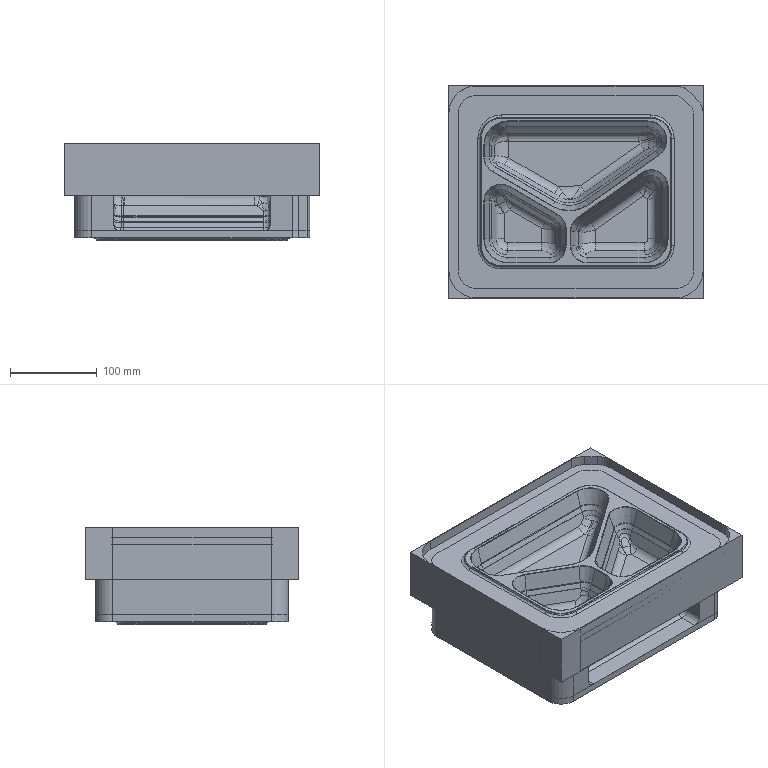NC program | NX | posted with a generic post | part box 295.651 x 246.652 x 112.895 mm
Lines 268779 to 269046 of 299251:
(D4 , TOOL : V2.0)
N537544 M6
N537546 G53
N537548 G17 G0 G90 X123.435 Y60.74 S2000 M3 M8
N537550 G43 Z210.5 H0
N537552 G94 G81 G98 Z46.884 F150. R51.884
N537554 X115.435 Y60.61
N537556 X113.468 Y72.487
N537558 X121.842 Y72.731
N537560 X116.481 Y83.572
N537562 X106.869 Y82.551
N537564 X107.906 Y92.1
N537566 X97.036 Y97.401
N537568 X96.748 Y89.06
N537570 X84.854 Y90.936
N537572 X85.037 Y98.936
N537574 X72.889
N537576 X72.732 Y90.936
N537578 X60.61
N537580 X60.74 Y98.936
N537582 X48.592
N537584 X48.488 Y90.936
N537586 X36.444 Y98.936
N537588 X36.366 Y90.936
N537590 X24.244
N537592 X24.296 Y98.936
N537594 X12.148
N537596 X12.122 Y90.936
N537598 X0.
N537600 Y98.936
N537602 X-12.148
N537604 X-12.122 Y90.936
N537606 X-24.244
N537608 X-24.296 Y98.936
N537610 X-36.444
N537612 X-36.366 Y90.936
N537614 X-48.488
N537616 X-48.592 Y98.936
N537618 X-60.74
N537620 X-72.889
N537622 X-85.037
N537624 X-84.854 Y90.936
N537626 X-96.748 Y89.06
N537628 X-97.036 Y97.401
N537630 X-107.906 Y92.1
N537632 X-106.869 Y82.551
N537634 X-116.481 Y83.572
N537636 X-121.842 Y72.731
N537638 X-113.468 Y72.487
N537640 X-106.216 Y70.651 Z50.395 R55.395
N537642 X-100.153 Y78.648
N537644 X-91.124 Y83.028
N537646 X-81.031 Y83.531
N537648 X-70.902
N537650 X-72.732 Y90.936 Z46.884 R51.884
N537652 X-60.61
N537654 X-60.773 Y83.531 Z50.395 R55.395
N537656 X-50.644
N537658 X-40.516
N537660 X-30.387
N537662 X-20.258
N537664 X-10.129
N537666 X0.
N537668 X10.129
N537670 X20.258
N537672 X30.387
N537674 X40.516
N537676 X50.644
N537678 X60.773
N537680 X70.902
N537682 X81.031
N537684 X91.124 Y83.028
N537686 X100.153 Y78.648
N537688 X106.216 Y70.651
N537690 X108.031 Y60.773
N537692 Y50.644
N537694 X115.435 Y48.488 Z46.884 R51.884
N537696 X123.435 Y48.592
N537698 Y36.444
N537700 X115.435 Y36.366
N537702 Y24.244
N537704 X123.435 Y24.296
N537706 Y12.148
N537708 X115.435 Y12.122
N537710 X108.031 Y10.129 Z50.395 R55.395
N537712 Y20.258
N537714 Y30.387
N537716 X103.561 Y30.537
N537718 X97.515 Y31.319
N537720 X108.031 Y40.516
N537722 X99.281 Y41.768
N537724 X90.53 Y35.641
N537726 X90.272 Y29.631
N537728 X81.78 Y29.515
N537730 X73.03 Y23.388
N537732 X64.28 Y17.261
N537734 X55.53 Y11.134
N537736 X46.78 Y5.007
N537738 X38.029 Y-1.12
N537740 X29.279 Y-7.247
N537742 X20.529 Y-13.374
N537744 X11.779 Y-19.501
N537746 X3.029 Y-25.628
N537748 X-5.721 Y-31.755
N537750 X-8.805 Y-29.974
N537752 Y-40.685
N537754 Y-51.397
N537756 Y-62.108
N537758 Y-72.82
N537760 X0. Y-83.531
N537762 X-10.129
N537764 X-20.258
N537766 X-30.387
N537768 X-40.516
N537770 X-50.644
N537772 X-60.773
N537774 X-70.902
N537776 X-81.031
N537778 X-91.124 Y-83.028
N537780 X-100.153 Y-78.648
N537782 X-106.216 Y-70.651
N537784 X-113.468 Y-72.487 Z46.884 R51.884
N537786 X-121.842 Y-72.731
N537788 X-116.481 Y-83.572
N537790 X-106.869 Y-82.551
N537792 X-107.906 Y-92.1
N537794 X-97.036 Y-97.401
N537796 X-96.748 Y-89.06
N537798 X-84.854 Y-90.936
N537800 X-85.037 Y-98.936
N537802 X-72.889
N537804 X-72.732 Y-90.936
N537806 X-60.61
N537808 X-60.74 Y-98.936
N537810 X-48.592
N537812 X-48.488 Y-90.936
N537814 X-36.444 Y-98.936
N537816 X-36.366 Y-90.936
N537818 X-24.244
N537820 X-24.296 Y-98.936
N537822 X-12.148
N537824 X-12.122 Y-90.936
N537826 X0.
N537828 Y-98.936
N537830 X12.148
N537832 X12.122 Y-90.936
N537834 X10.129 Y-83.531 Z50.395 R55.395
N537836 X20.258
N537838 X24.244 Y-90.936 Z46.884 R51.884
N537840 X24.296 Y-98.936
N537842 X30.387 Y-83.531 Z50.395 R55.395
N537844 X40.516
N537846 X50.644
N537848 X48.488 Y-90.936 Z46.884 R51.884
N537850 X36.366
N537852 X36.444 Y-98.936
N537854 X48.592
N537856 X60.74
N537858 X60.61 Y-90.936
N537860 X60.773 Y-83.531 Z50.395 R55.395
N537862 X70.902
N537864 X72.732 Y-90.936 Z46.884 R51.884
N537866 X72.889 Y-98.936
N537868 X85.037
N537870 X84.854 Y-90.936
N537872 X81.031 Y-83.531 Z50.395 R55.395
N537874 X91.124 Y-83.028
N537876 X100.153 Y-78.648
N537878 X96.748 Y-89.06 Z46.884 R51.884
N537880 X97.036 Y-97.401
N537882 X107.906 Y-92.1
N537884 X106.869 Y-82.551
N537886 X106.216 Y-70.651 Z50.395 R55.395
N537888 X113.468 Y-72.487 Z46.884 R51.884
N537890 X116.481 Y-83.572
N537892 X121.842 Y-72.731
N537894 X123.435 Y-60.74
N537896 X115.435 Y-60.61
N537898 X108.031 Y-60.773 Z50.395 R55.395
N537900 Y-50.644
N537902 X115.435 Y-48.488 Z46.884 R51.884
N537904 X123.435 Y-48.592
N537906 X115.435 Y-36.366
N537908 X123.435 Y-36.444
N537910 Y-24.296
N537912 X115.435 Y-24.244
N537914 Y-12.122
N537916 X123.435 Y-12.148
N537918 Y0.
N537920 X115.435
N537922 X108.031 Z50.395 R55.395
N537924 Y-10.129
N537926 Y-20.258
N537928 Y-30.387
N537930 Y-40.516
N537932 X83.46 Y-31.008 Z6.035 R11.035
N537934 X60.615 Y-44.511 Z6. R11.
N537936 X53.174 Y-58.227
N537938 X35.615 Y-44.511
N537940 X60.615 Y-19.511
N537942 X73.032 Y57.433
N537944 X48.032
N537946 X23.032
N537948 Y32.433
N537950 X-1.968
N537952 X-26.968
N537954 X-1.968 Y57.433
N537956 X-26.968
N537958 X-51.968
N537960 X-76.968
N537962 X-51.968 Y32.433
N537964 X-64.847 Y-27.339 Z6.007 R11.007
N537966 X-83.114 Y-39.521 Z6. R11.
N537968 X-64.847 Y-47.339
N537970 X-44.847
N537972 X-18.106 Y-24.604 Z50.395 R55.395
N537974 X-27.407 Y-19.234
N537976 X-36.708 Y-13.864
N537978 X-46.009 Y-8.495
N537980 X-55.31 Y-3.125
N537982 X-64.611 Y2.245
N537984 X-73.912 Y7.615
N537986 X-83.212 Y12.985
N537988 X-92.513 Y18.355
N537990 X-100.563 Y11.963
N537992 X-108.031 Y10.129
N537994 Y20.258
N537996 X-103.598 Y18.877
N537998 X-101.814 Y23.725
N538000 X-108.031 Y30.387
N538002 Y40.516
N538004 Y50.644
N538006 Y60.773
N538008 X-115.435 Y60.61 Z46.884 R51.884
N538010 X-123.435 Y60.74
N538012 Y48.592
N538014 X-115.435 Y48.488
N538016 Y36.366
N538018 X-123.435 Y36.444
N538020 Y24.296
N538022 X-115.435 Y24.244
N538024 Y12.122
N538026 X-123.435 Y12.148
N538028 Y0.
N538030 X-115.435
N538032 X-108.031 Z50.395 R55.395
N538034 Y-10.129
N538036 Y-20.258
N538038 Y-30.387
N538040 Y-40.516
N538042 Y-50.644
N538044 Y-60.773
N538046 X-115.435 Y-60.61 Z46.884 R51.884
N538048 X-123.435 Y-60.74
N538050 Y-48.592
N538052 X-115.435 Y-48.488
N538054 Y-36.366
N538056 X-123.435 Y-36.444
N538058 Y-24.296
N538060 X-115.435 Y-24.244
N538062 Y-12.122
N538064 X-123.435 Y-12.148
N538066 G80
N538068 G0 X-123.435 Y-12.148 Z210.5
N538070 M9
N538072 M5